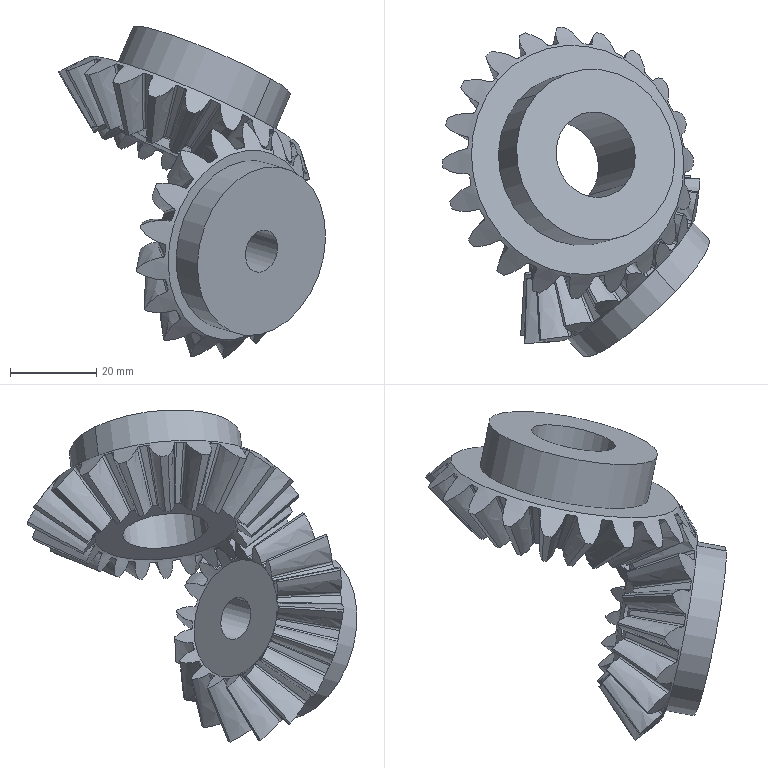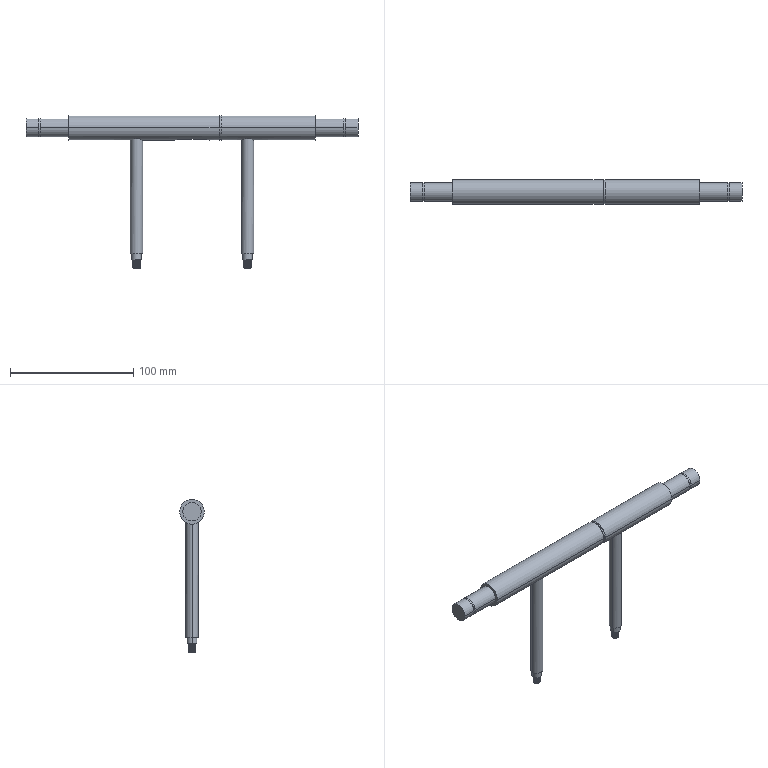Simulation study | ansys workbench
Set-up summary:
category,name,step,type,value,unit,region
solver,ansys_mapdl
solver,version,,,22.1
solver,version,,,22.1
solver,version,,,22.1
units,MPA,,stated
analysis,deck1,,static,static
load_step,requested,,,1
analysis,nlgeom,,,False
mesh,nodes,,,35715
mesh,elements,,,25058
element_type,ANSYS 187 (type 1),,solid,5799
element_type,ANSYS 187 (type 2),,solid,8098
element_type,ANSYS 187 (type 3),,solid,5799
element_type,ANSYS 174 (type 4),,contact,1445
element_type,ANSYS 170 (type 5),,target,1445
element_type,ANSYS 174 (type 6),,contact,1038
element_type,ANSYS 170 (type 7),,target,1038
element_type,ANSYS 174 (type 8),,contact,396
element_type,ANSYS 170 (type 9),,target,0
load,load commands in deck,,count,3
bc,support commands in deck,,count,1
named_set,_FIXEDSU,,component
analysis,deck2,,static,static
load_step,requested,,,1
analysis,nlgeom,,,False
mesh,nodes,,,3352
mesh,elements,,,2009
element_type,ANSYS 187 (type 1),,solid,1603
element_type,ANSYS 154 (type 2),,surface,406
load,load commands in deck,,count,3
bc,support commands in deck,,count,1
named_set,_FIXEDSU,,component
analysis,deck3,,static,static
load_step,requested,,,1
analysis,nlgeom,,,False
mesh,nodes,,,31828
mesh,elements,,,18520
element_type,ANSYS 187 (type 1),,solid,8110
element_type,ANSYS 187 (type 2),,solid,9496
element_type,ANSYS 174 (type 3),,contact,276
element_type,ANSYS 170 (type 4),,target,276
element_type,ANSYS 174 (type 5),,contact,362
element_type,ANSYS 170 (type 6),,target,0
load,load commands in deck,,count,3
bc,support commands in deck,,count,1
named_set,_FIXEDSU,,component
material,1,,in results
material,2,,in results
material,3,,in results
material,1,,in results
material,1,,in results
material,2,,in results
check,setup vs results,,match,results also hold 1 node(s) and 1 element(s) the deck makes with ['EN']; those were not compared
check,setup vs results,,match,406 surface effect element(s) are not in the reader's mesh and were not compared
check,setup vs results,,match,results also hold 1 node(s) and 1 element(s) the deck makes with ['EN']; those were not compared
Results summary:
result,analysis,,,static
result,last_loadstep,,,1
result,primary field,,,displacement
result,reaction total,1,FX,-0.0,N
result,reaction total,1,FY,-0.0,N
result,reaction total,1,FZ,-0.0,N
result,mass,,,0.000693,"NMM: mm, ton, N, s, mV, mA, degC"
result,analysis,,,static
result,last_loadstep,,,1
result,primary field,,,displacement
result,reaction total,1,FX,-0.0,N
result,reaction total,1,FY,500.0,N
result,reaction total,1,FZ,-0.0,N
result,mass,,,0.007291,"NMM: mm, ton, N, s, mV, mA, degC"
result,analysis,,,static
result,last_loadstep,,,1
result,primary field,,,displacement
result,reaction total,1,FX,-0.0,N
result,reaction total,1,FY,-0.0,N
result,reaction total,1,FZ,-0.0,N
result,mass,,,0.000453,"NMM: mm, ton, N, s, mV, mA, degC"